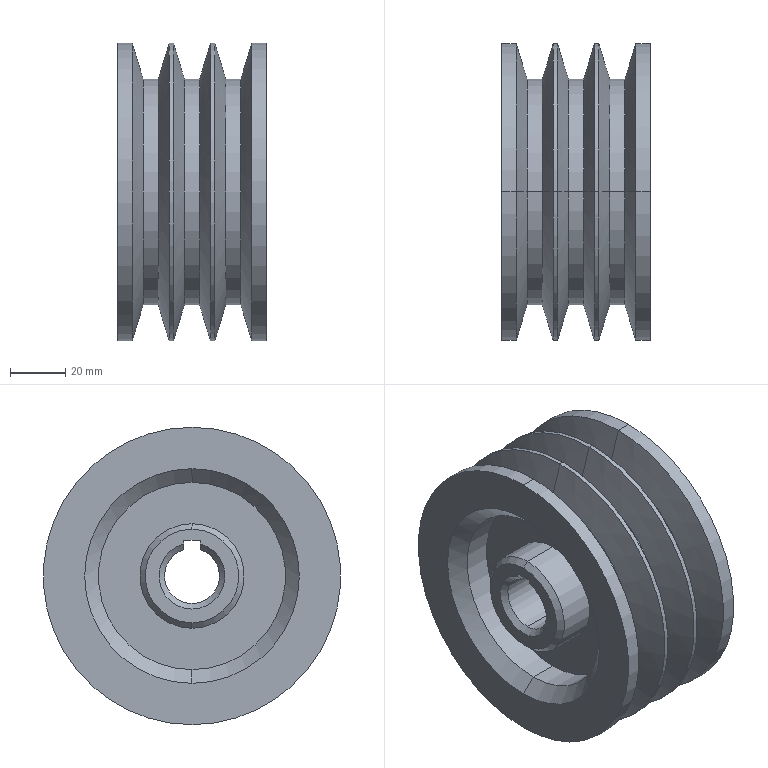Part | STEP file | Driven pulley | 1 solid | 54 faces | box 54 x 108 x 108 mm | volume 283345 mm3 | cylinder 24 | cone 21 | plane 9 | commonest cylinder face diameters 108 x8 82 x6 38 x4 68 x4 20 x2
STEP:
#1=CARTESIAN_POINT('',(17.5,0.,-10.));
#2=VERTEX_POINT('',#1);
#3=CARTESIAN_POINT('',(17.5,3.,9.539));
#4=VERTEX_POINT('',#3);
#5=CARTESIAN_POINT('',(17.5,0.,0.));
#6=DIRECTION('',(1.,0.,0.));
#7=DIRECTION('',(0.,0.,1.));
#8=AXIS2_PLACEMENT_3D('',#5,#6,#7);
#9=CIRCLE('',#8,10.);
#10=EDGE_CURVE('',#2,#4,#9,.T.);
#11=ORIENTED_EDGE('',*,*,#10,.F.);
#12=CARTESIAN_POINT('',(19.5,0.,-12.));
#13=VERTEX_POINT('',#12);
#14=CARTESIAN_POINT('',(17.5,0.,-10.));
#15=DIRECTION('',(0.7071,0.,-0.7071));
#16=VECTOR('',#15,1000.);
#17=LINE('',#14,#16);
#18=EDGE_CURVE('',#2,#13,#17,.T.);
#19=ORIENTED_EDGE('',*,*,#18,.T.);
#20=CARTESIAN_POINT('',(19.5,3.,11.619));
#21=VERTEX_POINT('',#20);
#22=CARTESIAN_POINT('',(19.5,0.,0.));
#23=DIRECTION('',(-1.,0.,0.));
#24=DIRECTION('',(0.,0.,1.));
#25=AXIS2_PLACEMENT_3D('',#22,#23,#24);
#26=CIRCLE('',#25,12.);
#27=EDGE_CURVE('',#21,#13,#26,.T.);
#28=ORIENTED_EDGE('',*,*,#27,.F.);
#29=CARTESIAN_POINT('',(17.5,3.,9.539));
#30=CARTESIAN_POINT('',(18.164,3.,10.235));
#31=CARTESIAN_POINT('',(18.831,3.,10.928));
#32=CARTESIAN_POINT('',(19.5,3.,11.619));
#33=B_SPLINE_CURVE_WITH_KNOTS('',3,(#29,#30,#31,#32),.UNSPECIFIED.,.F.,.F.,(4,4),(0.,0.002885),.UNSPECIFIED.);
#34=EDGE_CURVE('',#4,#21,#33,.T.);
#35=ORIENTED_EDGE('',*,*,#34,.F.);
#36=EDGE_LOOP('',(#11,#19,#28,#35));
#37=FACE_OUTER_BOUND('',#36,.T.);
#38=CARTESIAN_POINT('',(17.5,0.,0.));
#39=DIRECTION('',(1.,0.,0.));
#40=DIRECTION('',(0.,0.,-1.));
#41=AXIS2_PLACEMENT_3D('',#38,#39,#40);
#42=CONICAL_SURFACE('',#41,10.,0.7854);
#43=ADVANCED_FACE('',(#37),#42,.F.);
#44=CARTESIAN_POINT('',(-34.5,0.,17.));
#45=VERTEX_POINT('',#44);
#46=CARTESIAN_POINT('',(-34.5,0.,-17.));
#47=VERTEX_POINT('',#46);
#48=CARTESIAN_POINT('',(-34.5,0.,0.));
#49=DIRECTION('',(-1.,0.,0.));
#50=DIRECTION('',(0.,0.,-1.));
#51=AXIS2_PLACEMENT_3D('',#48,#49,#50);
#52=CIRCLE('',#51,17.);
#53=EDGE_CURVE('',#45,#47,#52,.T.);
#54=ORIENTED_EDGE('',*,*,#53,.F.);
#55=CARTESIAN_POINT('',(-32.5,0.,19.));
#56=VERTEX_POINT('',#55);
#57=CARTESIAN_POINT('',(-34.5,0.,17.));
#58=DIRECTION('',(0.7071,0.,0.7071));
#59=VECTOR('',#58,1000.);
#60=LINE('',#57,#59);
#61=EDGE_CURVE('',#45,#56,#60,.T.);
#62=ORIENTED_EDGE('',*,*,#61,.T.);
#63=CARTESIAN_POINT('',(-32.5,0.,-19.));
#64=VERTEX_POINT('',#63);
#65=CARTESIAN_POINT('',(-32.5,0.,0.));
#66=DIRECTION('',(1.,0.,0.));
#67=DIRECTION('',(0.,0.,-1.));
#68=AXIS2_PLACEMENT_3D('',#65,#66,#67);
#69=CIRCLE('',#68,19.);
#70=EDGE_CURVE('',#64,#56,#69,.T.);
#71=ORIENTED_EDGE('',*,*,#70,.F.);
#72=CARTESIAN_POINT('',(-34.5,0.,-17.));
#73=DIRECTION('',(0.7071,0.,-0.7071));
#74=VECTOR('',#73,1000.);
#75=LINE('',#72,#74);
#76=EDGE_CURVE('',#47,#64,#75,.T.);
#77=ORIENTED_EDGE('',*,*,#76,.F.);
#78=EDGE_LOOP('',(#54,#62,#71,#77));
#79=FACE_OUTER_BOUND('',#78,.T.);
#80=CARTESIAN_POINT('',(-34.5,0.,0.));
#81=DIRECTION('',(1.,0.,0.));
#82=DIRECTION('',(0.,0.,-1.));
#83=AXIS2_PLACEMENT_3D('',#80,#81,#82);
#84=CONICAL_SURFACE('',#83,17.,0.7854);
#85=ADVANCED_FACE('',(#79),#84,.T.);
#86=CARTESIAN_POINT('',(14.5,0.,34.));
#87=VERTEX_POINT('',#86);
#88=CARTESIAN_POINT('',(14.5,0.,-34.));
#89=VERTEX_POINT('',#88);
#90=CARTESIAN_POINT('',(14.5,0.,0.));
#91=DIRECTION('',(1.,0.,0.));
#92=DIRECTION('',(0.,0.,1.));
#93=AXIS2_PLACEMENT_3D('',#90,#91,#92);
#94=CIRCLE('',#93,34.);
#95=EDGE_CURVE('',#87,#89,#94,.T.);
#96=ORIENTED_EDGE('',*,*,#95,.F.);
#97=CARTESIAN_POINT('',(19.5,0.,39.));
#98=VERTEX_POINT('',#97);
#99=CARTESIAN_POINT('',(19.5,0.,39.));
#100=DIRECTION('',(0.7071,0.,0.7071));
#101=VECTOR('',#100,1000.);
#102=LINE('',#99,#101);
#103=EDGE_CURVE('',#87,#98,#102,.T.);
#104=ORIENTED_EDGE('',*,*,#103,.T.);
#105=CARTESIAN_POINT('',(19.5,0.,-39.));
#106=VERTEX_POINT('',#105);
#107=CARTESIAN_POINT('',(19.5,0.,0.));
#108=DIRECTION('',(-1.,0.,0.));
#109=DIRECTION('',(0.,0.,1.));
#110=AXIS2_PLACEMENT_3D('',#107,#108,#109);
#111=CIRCLE('',#110,39.);
#112=EDGE_CURVE('',#106,#98,#111,.T.);
#113=ORIENTED_EDGE('',*,*,#112,.F.);
#114=CARTESIAN_POINT('',(19.5,0.,-39.));
#115=DIRECTION('',(0.7071,0.,-0.7071));
#116=VECTOR('',#115,1000.);
#117=LINE('',#114,#116);
#118=EDGE_CURVE('',#89,#106,#117,.T.);
#119=ORIENTED_EDGE('',*,*,#118,.F.);
#120=EDGE_LOOP('',(#96,#104,#113,#119));
#121=FACE_OUTER_BOUND('',#120,.T.);
#122=CARTESIAN_POINT('',(19.5,0.,0.));
#123=DIRECTION('',(1.,0.,0.));
#124=DIRECTION('',(0.,0.,-1.));
#125=AXIS2_PLACEMENT_3D('',#122,#123,#124);
#126=CONICAL_SURFACE('',#125,39.,0.7854);
#127=ADVANCED_FACE('',(#121),#126,.F.);
#128=CARTESIAN_POINT('',(-29.5,0.,-34.));
#129=VERTEX_POINT('',#128);
#130=CARTESIAN_POINT('',(-29.5,0.,34.));
#131=VERTEX_POINT('',#130);
#132=CARTESIAN_POINT('',(-29.5,0.,0.));
#133=DIRECTION('',(-1.,0.,0.));
#134=DIRECTION('',(0.,0.,-1.));
#135=AXIS2_PLACEMENT_3D('',#132,#133,#134);
#136=CIRCLE('',#135,34.);
#137=EDGE_CURVE('',#129,#131,#136,.T.);
#138=ORIENTED_EDGE('',*,*,#137,.F.);
#139=CARTESIAN_POINT('',(-34.5,0.,-39.));
#140=VERTEX_POINT('',#139);
#141=CARTESIAN_POINT('',(-29.5,0.,-34.));
#142=DIRECTION('',(-0.7071,0.,-0.7071));
#143=VECTOR('',#142,1000.);
#144=LINE('',#141,#143);
#145=EDGE_CURVE('',#129,#140,#144,.T.);
#146=ORIENTED_EDGE('',*,*,#145,.T.);
#147=CARTESIAN_POINT('',(-34.5,0.,39.));
#148=VERTEX_POINT('',#147);
#149=CARTESIAN_POINT('',(-34.5,0.,0.));
#150=DIRECTION('',(1.,0.,0.));
#151=DIRECTION('',(0.,0.,-1.));
#152=AXIS2_PLACEMENT_3D('',#149,#150,#151);
#153=CIRCLE('',#152,39.);
#154=EDGE_CURVE('',#148,#140,#153,.T.);
#155=ORIENTED_EDGE('',*,*,#154,.F.);
#156=CARTESIAN_POINT('',(-29.5,0.,34.));
#157=DIRECTION('',(-0.7071,0.,0.7071));
#158=VECTOR('',#157,1000.);
#159=LINE('',#156,#158);
#160=EDGE_CURVE('',#131,#148,#159,.T.);
#161=ORIENTED_EDGE('',*,*,#160,.F.);
#162=EDGE_LOOP('',(#138,#146,#155,#161));
#163=FACE_OUTER_BOUND('',#162,.T.);
#164=CARTESIAN_POINT('',(-29.5,0.,0.));
#165=DIRECTION('',(-1.,0.,0.));
#166=DIRECTION('',(0.,0.,1.));
#167=AXIS2_PLACEMENT_3D('',#164,#165,#166);
#168=CONICAL_SURFACE('',#167,34.,0.7854);
#169=ADVANCED_FACE('',(#163),#168,.F.);
#170=CARTESIAN_POINT('',(4.5,0.,19.));
#171=VERTEX_POINT('',#170);
#172=CARTESIAN_POINT('',(4.5,0.,-19.));
#173=VERTEX_POINT('',#172);
#174=CARTESIAN_POINT('',(4.5,0.,0.));
#175=DIRECTION('',(-1.,0.,0.));
#176=DIRECTION('',(0.,0.,1.));
#177=AXIS2_PLACEMENT_3D('',#174,#175,#176);
#178=CIRCLE('',#177,19.);
#179=EDGE_CURVE('',#171,#173,#178,.T.);
#180=ORIENTED_EDGE('',*,*,#179,.F.);
#181=CARTESIAN_POINT('',(19.5,0.,19.));
#182=VERTEX_POINT('',#181);
#183=CARTESIAN_POINT('',(4.5,0.,19.));
#184=DIRECTION('',(1.,0.,0.));
#185=VECTOR('',#184,1000.);
#186=LINE('',#183,#185);
#187=EDGE_CURVE('',#171,#182,#186,.T.);
#188=ORIENTED_EDGE('',*,*,#187,.T.);
#189=CARTESIAN_POINT('',(19.5,0.,-19.));
#190=VERTEX_POINT('',#189);
#191=CARTESIAN_POINT('',(19.5,0.,0.));
#192=DIRECTION('',(-1.,0.,0.));
#193=DIRECTION('',(0.,0.,1.));
#194=AXIS2_PLACEMENT_3D('',#191,#192,#193);
#195=CIRCLE('',#194,19.);
#196=EDGE_CURVE('',#182,#190,#195,.T.);
#197=ORIENTED_EDGE('',*,*,#196,.T.);
#198=CARTESIAN_POINT('',(4.5,0.,-19.));
#199=DIRECTION('',(1.,0.,0.));
#200=VECTOR('',#199,1000.);
#201=LINE('',#198,#200);
#202=EDGE_CURVE('',#173,#190,#201,.T.);
#203=ORIENTED_EDGE('',*,*,#202,.F.);
#204=EDGE_LOOP('',(#180,#188,#197,#203));
#205=FACE_OUTER_BOUND('',#204,.T.);
#206=CARTESIAN_POINT('',(4.5,0.,0.));
#207=DIRECTION('',(1.,0.,0.));
#208=DIRECTION('',(0.,0.,-1.));
#209=AXIS2_PLACEMENT_3D('',#206,#207,#208);
#210=CYLINDRICAL_SURFACE('',#209,19.);
#211=ADVANCED_FACE('',(#205),#210,.T.);
#212=CARTESIAN_POINT('',(4.5,0.,-34.));
#213=VERTEX_POINT('',#212);
#214=CARTESIAN_POINT('',(4.5,0.,34.));
#215=VERTEX_POINT('',#214);
#216=CARTESIAN_POINT('',(4.5,0.,0.));
#217=DIRECTION('',(-1.,0.,0.));
#218=DIRECTION('',(0.,0.,1.));
#219=AXIS2_PLACEMENT_3D('',#216,#217,#218);
#220=CIRCLE('',#219,34.);
#221=EDGE_CURVE('',#213,#215,#220,.T.);
#222=ORIENTED_EDGE('',*,*,#221,.T.);
#223=CARTESIAN_POINT('',(4.5,0.,34.));
#224=DIRECTION('',(1.,0.,0.));
#225=VECTOR('',#224,1000.);
#226=LINE('',#223,#225);
#227=EDGE_CURVE('',#215,#87,#226,.T.);
#228=ORIENTED_EDGE('',*,*,#227,.T.);
#229=ORIENTED_EDGE('',*,*,#95,.T.);
#230=CARTESIAN_POINT('',(4.5,0.,-34.));
#231=DIRECTION('',(1.,0.,0.));
#232=VECTOR('',#231,1000.);
#233=LINE('',#230,#232);
#234=EDGE_CURVE('',#213,#89,#233,.T.);
#235=ORIENTED_EDGE('',*,*,#234,.F.);
#236=EDGE_LOOP('',(#222,#228,#229,#235));
#237=FACE_OUTER_BOUND('',#236,.T.);
#238=CARTESIAN_POINT('',(4.5,0.,0.));
#239=DIRECTION('',(1.,0.,0.));
#240=DIRECTION('',(0.,0.,-1.));
#241=AXIS2_PLACEMENT_3D('',#238,#239,#240);
#242=CYLINDRICAL_SURFACE('',#241,34.);
#243=ADVANCED_FACE('',(#237),#242,.F.);
#244=CARTESIAN_POINT('',(-19.5,0.,19.));
#245=VERTEX_POINT('',#244);
#246=CARTESIAN_POINT('',(-19.5,0.,-19.));
#247=VERTEX_POINT('',#246);
#248=CARTESIAN_POINT('',(-19.5,0.,0.));
#249=DIRECTION('',(-1.,0.,0.));
#250=DIRECTION('',(0.,0.,1.));
#251=AXIS2_PLACEMENT_3D('',#248,#249,#250);
#252=CIRCLE('',#251,19.);
#253=EDGE_CURVE('',#245,#247,#252,.T.);
#254=ORIENTED_EDGE('',*,*,#253,.T.);
#255=CARTESIAN_POINT('',(-19.5,0.,-19.));
#256=DIRECTION('',(-1.,0.,0.));
#257=VECTOR('',#256,1000.);
#258=LINE('',#255,#257);
#259=EDGE_CURVE('',#247,#64,#258,.T.);
#260=ORIENTED_EDGE('',*,*,#259,.T.);
#261=ORIENTED_EDGE('',*,*,#70,.T.);
#262=CARTESIAN_POINT('',(-19.5,0.,19.));
#263=DIRECTION('',(-1.,0.,0.));
#264=VECTOR('',#263,1000.);
#265=LINE('',#262,#264);
#266=EDGE_CURVE('',#245,#56,#265,.T.);
#267=ORIENTED_EDGE('',*,*,#266,.F.);
#268=EDGE_LOOP('',(#254,#260,#261,#267));
#269=FACE_OUTER_BOUND('',#268,.T.);
#270=CARTESIAN_POINT('',(-19.5,0.,0.));
#271=DIRECTION('',(-1.,0.,0.));
#272=DIRECTION('',(0.,0.,1.));
#273=AXIS2_PLACEMENT_3D('',#270,#271,#272);
#274=CYLINDRICAL_SURFACE('',#273,19.);
#275=ADVANCED_FACE('',(#269),#274,.T.);
#276=CARTESIAN_POINT('',(-19.5,0.,-34.));
#277=VERTEX_POINT('',#276);
#278=CARTESIAN_POINT('',(-19.5,0.,34.));
#279=VERTEX_POINT('',#278);
#280=CARTESIAN_POINT('',(-19.5,0.,0.));
#281=DIRECTION('',(-1.,0.,0.));
#282=DIRECTION('',(0.,0.,1.));
#283=AXIS2_PLACEMENT_3D('',#280,#281,#282);
#284=CIRCLE('',#283,34.);
#285=EDGE_CURVE('',#277,#279,#284,.T.);
#286=ORIENTED_EDGE('',*,*,#285,.F.);
#287=CARTESIAN_POINT('',(-19.5,0.,-34.));
#288=DIRECTION('',(-1.,0.,0.));
#289=VECTOR('',#288,1000.);
#290=LINE('',#287,#289);
#291=EDGE_CURVE('',#277,#129,#290,.T.);
#292=ORIENTED_EDGE('',*,*,#291,.T.);
#293=ORIENTED_EDGE('',*,*,#137,.T.);
#294=CARTESIAN_POINT('',(-19.5,0.,34.));
#295=DIRECTION('',(-1.,0.,0.));
#296=VECTOR('',#295,1000.);
#297=LINE('',#294,#296);
#298=EDGE_CURVE('',#279,#131,#297,.T.);
#299=ORIENTED_EDGE('',*,*,#298,.F.);
#300=EDGE_LOOP('',(#286,#292,#293,#299));
#301=FACE_OUTER_BOUND('',#300,.T.);
#302=CARTESIAN_POINT('',(-19.5,0.,0.));
#303=DIRECTION('',(-1.,0.,0.));
#304=DIRECTION('',(0.,0.,1.));
#305=AXIS2_PLACEMENT_3D('',#302,#303,#304);
#306=CYLINDRICAL_SURFACE('',#305,34.);
#307=ADVANCED_FACE('',(#301),#306,.F.);
#308=CARTESIAN_POINT('',(-32.5,3.,9.539));
#309=VERTEX_POINT('',#308);
#310=CARTESIAN_POINT('',(-32.5,0.,-10.));
#311=VERTEX_POINT('',#310);
#312=CARTESIAN_POINT('',(-32.5,0.,0.));
#313=DIRECTION('',(-1.,0.,0.));
#314=DIRECTION('',(0.,0.,-1.));
#315=AXIS2_PLACEMENT_3D('',#312,#313,#314);
#316=CIRCLE('',#315,10.);
#317=EDGE_CURVE('',#309,#311,#316,.T.);
#318=ORIENTED_EDGE('',*,*,#317,.T.);
#319=CARTESIAN_POINT('',(-59.5,0.,-10.));
#320=DIRECTION('',(1.,0.,0.));
#321=VECTOR('',#320,1000.);
#322=LINE('',#319,#321);
#323=EDGE_CURVE('',#311,#2,#322,.T.);
#324=ORIENTED_EDGE('',*,*,#323,.T.);
#325=ORIENTED_EDGE('',*,*,#10,.T.);
#326=CARTESIAN_POINT('',(-59.5,3.,9.539));
#327=DIRECTION('',(-1.,0.,0.));
#328=VECTOR('',#327,1000.);
#329=LINE('',#326,#328);
#330=EDGE_CURVE('',#4,#309,#329,.T.);
#331=ORIENTED_EDGE('',*,*,#330,.T.);
#332=EDGE_LOOP('',(#318,#324,#325,#331));
#333=FACE_OUTER_BOUND('',#332,.T.);
#334=CARTESIAN_POINT('',(-59.5,0.,0.));
#335=DIRECTION('',(1.,0.,0.));
#336=DIRECTION('',(0.,0.,-1.));
#337=AXIS2_PLACEMENT_3D('',#334,#335,#336);
#338=CYLINDRICAL_SURFACE('',#337,10.);
#339=ADVANCED_FACE('',(#333),#338,.F.);
#340=CARTESIAN_POINT('',(19.5,0.,54.));
#341=VERTEX_POINT('',#340);
#342=CARTESIAN_POINT('',(19.5,0.,-54.));
#343=VERTEX_POINT('',#342);
#344=CARTESIAN_POINT('',(19.5,0.,0.));
#345=DIRECTION('',(-1.,0.,0.));
#346=DIRECTION('',(0.,0.,1.));
#347=AXIS2_PLACEMENT_3D('',#344,#345,#346);
#348=CIRCLE('',#347,54.);
#349=EDGE_CURVE('',#341,#343,#348,.T.);
#350=ORIENTED_EDGE('',*,*,#349,.T.);
#351=CARTESIAN_POINT('',(14.223,0.,-54.));
#352=VERTEX_POINT('',#351);
#353=CARTESIAN_POINT('',(0.,0.,-54.));
#354=DIRECTION('',(-1.,0.,0.));
#355=VECTOR('',#354,1000.);
#356=LINE('',#353,#355);
#357=EDGE_CURVE('',#343,#352,#356,.T.);
#358=ORIENTED_EDGE('',*,*,#357,.T.);
#359=CARTESIAN_POINT('',(14.223,0.,54.));
#360=VERTEX_POINT('',#359);
#361=CARTESIAN_POINT('',(14.223,0.,0.));
#362=DIRECTION('',(-1.,0.,0.));
#363=DIRECTION('',(0.,0.,1.));
#364=AXIS2_PLACEMENT_3D('',#361,#362,#363);
#365=CIRCLE('',#364,54.);
#366=EDGE_CURVE('',#360,#352,#365,.T.);
#367=ORIENTED_EDGE('',*,*,#366,.F.);
#368=CARTESIAN_POINT('',(0.,0.,54.));
#369=DIRECTION('',(-1.,0.,0.));
#370=VECTOR('',#369,1000.);
#371=LINE('',#368,#370);
#372=EDGE_CURVE('',#341,#360,#371,.T.);
#373=ORIENTED_EDGE('',*,*,#372,.F.);
#374=EDGE_LOOP('',(#350,#358,#367,#373));
#375=FACE_OUTER_BOUND('',#374,.T.);
#376=CARTESIAN_POINT('',(0.,0.,0.));
#377=DIRECTION('',(-1.,0.,0.));
#378=DIRECTION('',(0.,0.,1.));
#379=AXIS2_PLACEMENT_3D('',#376,#377,#378);
#380=CYLINDRICAL_SURFACE('',#379,54.);
#381=ADVANCED_FACE('',(#375),#380,.T.);
#382=CARTESIAN_POINT('',(10.248,0.,41.));
#383=VERTEX_POINT('',#382);
#384=CARTESIAN_POINT('',(10.248,0.,-41.));
#385=VERTEX_POINT('',#384);
#386=CARTESIAN_POINT('',(10.248,0.,0.));
#387=DIRECTION('',(-1.,0.,0.));
#388=DIRECTION('',(0.,0.,1.));
#389=AXIS2_PLACEMENT_3D('',#386,#387,#388);
#390=CIRCLE('',#389,41.);
#391=EDGE_CURVE('',#383,#385,#390,.T.);
#392=ORIENTED_EDGE('',*,*,#391,.F.);
#393=CARTESIAN_POINT('',(14.223,0.,54.));
#394=DIRECTION('',(0.2924,0.,0.9563));
#395=VECTOR('',#394,1000.);
#396=LINE('',#393,#395);
#397=EDGE_CURVE('',#383,#360,#396,.T.);
#398=ORIENTED_EDGE('',*,*,#397,.T.);
#399=ORIENTED_EDGE('',*,*,#366,.T.);
#400=CARTESIAN_POINT('',(14.223,0.,-54.));
#401=DIRECTION('',(0.2924,0.,-0.9563));
#402=VECTOR('',#401,1000.);
#403=LINE('',#400,#402);
#404=EDGE_CURVE('',#385,#352,#403,.T.);
#405=ORIENTED_EDGE('',*,*,#404,.F.);
#406=EDGE_LOOP('',(#392,#398,#399,#405));
#407=FACE_OUTER_BOUND('',#406,.T.);
#408=CARTESIAN_POINT('',(14.223,0.,0.));
#409=DIRECTION('',(1.,0.,0.));
#410=DIRECTION('',(0.,0.,-1.));
#411=AXIS2_PLACEMENT_3D('',#408,#409,#410);
#412=CONICAL_SURFACE('',#411,54.,1.274);
#413=ADVANCED_FACE('',(#407),#412,.T.);
#414=ORIENTED_EDGE('',*,*,#391,.T.);
#415=CARTESIAN_POINT('',(4.752,0.,-41.));
#416=VERTEX_POINT('',#415);
#417=CARTESIAN_POINT('',(0.,0.,-41.));
#418=DIRECTION('',(-1.,0.,0.));
#419=VECTOR('',#418,1000.);
#420=LINE('',#417,#419);
#421=EDGE_CURVE('',#385,#416,#420,.T.);
#422=ORIENTED_EDGE('',*,*,#421,.T.);
#423=CARTESIAN_POINT('',(4.752,0.,41.));
#424=VERTEX_POINT('',#423);
#425=CARTESIAN_POINT('',(4.752,0.,0.));
#426=DIRECTION('',(-1.,0.,0.));
#427=DIRECTION('',(0.,0.,1.));
#428=AXIS2_PLACEMENT_3D('',#425,#426,#427);
#429=CIRCLE('',#428,41.);
#430=EDGE_CURVE('',#424,#416,#429,.T.);
#431=ORIENTED_EDGE('',*,*,#430,.F.);
#432=CARTESIAN_POINT('',(0.,0.,41.));
#433=DIRECTION('',(-1.,0.,0.));
#434=VECTOR('',#433,1000.);
#435=LINE('',#432,#434);
#436=EDGE_CURVE('',#383,#424,#435,.T.);
#437=ORIENTED_EDGE('',*,*,#436,.F.);
#438=EDGE_LOOP('',(#414,#422,#431,#437));
#439=FACE_OUTER_BOUND('',#438,.T.);
#440=CARTESIAN_POINT('',(0.,0.,0.));
#441=DIRECTION('',(-1.,0.,0.));
#442=DIRECTION('',(0.,0.,1.));
#443=AXIS2_PLACEMENT_3D('',#440,#441,#442);
#444=CYLINDRICAL_SURFACE('',#443,41.);
#445=ADVANCED_FACE('',(#439),#444,.T.);
#446=ORIENTED_EDGE('',*,*,#430,.T.);
#447=CARTESIAN_POINT('',(0.7771,0.,-54.));
#448=VERTEX_POINT('',#447);
#449=CARTESIAN_POINT('',(4.752,0.,-41.));
#450=DIRECTION('',(-0.2924,0.,-0.9563));
#451=VECTOR('',#450,1000.);
#452=LINE('',#449,#451);
#453=EDGE_CURVE('',#416,#448,#452,.T.);
#454=ORIENTED_EDGE('',*,*,#453,.T.);
#455=CARTESIAN_POINT('',(0.7771,0.,54.));
#456=VERTEX_POINT('',#455);
#457=CARTESIAN_POINT('',(0.7771,0.,0.));
#458=DIRECTION('',(-1.,0.,0.));
#459=DIRECTION('',(0.,0.,1.));
#460=AXIS2_PLACEMENT_3D('',#457,#458,#459);
#461=CIRCLE('',#460,54.);
#462=EDGE_CURVE('',#456,#448,#461,.T.);
#463=ORIENTED_EDGE('',*,*,#462,.F.);
#464=CARTESIAN_POINT('',(4.752,0.,41.));
#465=DIRECTION('',(-0.2924,0.,0.9563));
#466=VECTOR('',#465,1000.);
#467=LINE('',#464,#466);
#468=EDGE_CURVE('',#424,#456,#467,.T.);
#469=ORIENTED_EDGE('',*,*,#468,.F.);
#470=EDGE_LOOP('',(#446,#454,#463,#469));
#471=FACE_OUTER_BOUND('',#470,.T.);
#472=CARTESIAN_POINT('',(4.752,0.,0.));
#473=DIRECTION('',(-1.,0.,0.));
#474=DIRECTION('',(0.,0.,1.));
#475=AXIS2_PLACEMENT_3D('',#472,#473,#474);
#476=CONICAL_SURFACE('',#475,41.,1.274);
#477=ADVANCED_FACE('',(#471),#476,.T.);
#478=ORIENTED_EDGE('',*,*,#462,.T.);
#479=CARTESIAN_POINT('',(-0.7771,0.,-54.));
#480=VERTEX_POINT('',#479);
#481=CARTESIAN_POINT('',(0.,0.,-54.));
#482=DIRECTION('',(-1.,0.,0.));
#483=VECTOR('',#482,1000.);
#484=LINE('',#481,#483);
#485=EDGE_CURVE('',#448,#480,#484,.T.);
#486=ORIENTED_EDGE('',*,*,#485,.T.);
#487=CARTESIAN_POINT('',(-0.7771,0.,54.));
#488=VERTEX_POINT('',#487);
#489=CARTESIAN_POINT('',(-0.7771,0.,0.));
#490=DIRECTION('',(-1.,0.,0.));
#491=DIRECTION('',(0.,0.,1.));
#492=AXIS2_PLACEMENT_3D('',#489,#490,#491);
#493=CIRCLE('',#492,54.);
#494=EDGE_CURVE('',#488,#480,#493,.T.);
#495=ORIENTED_EDGE('',*,*,#494,.F.);
#496=CARTESIAN_POINT('',(0.,0.,54.));
#497=DIRECTION('',(-1.,0.,0.));
#498=VECTOR('',#497,1000.);
#499=LINE('',#496,#498);
#500=EDGE_CURVE('',#456,#488,#499,.T.);
#501=ORIENTED_EDGE('',*,*,#500,.F.);
#502=EDGE_LOOP('',(#478,#486,#495,#501));
#503=FACE_OUTER_BOUND('',#502,.T.);
#504=CARTESIAN_POINT('',(0.,0.,0.));
#505=DIRECTION('',(-1.,0.,0.));
#506=DIRECTION('',(0.,0.,1.));
#507=AXIS2_PLACEMENT_3D('',#504,#505,#506);
#508=CYLINDRICAL_SURFACE('',#507,54.);
#509=ADVANCED_FACE('',(#503),#508,.T.);
#510=CARTESIAN_POINT('',(-4.752,0.,41.));
#511=VERTEX_POINT('',#510);
#512=CARTESIAN_POINT('',(-4.752,0.,-41.));
#513=VERTEX_POINT('',#512);
#514=CARTESIAN_POINT('',(-4.752,0.,0.));
#515=DIRECTION('',(-1.,0.,0.));
#516=DIRECTION('',(0.,0.,1.));
#517=AXIS2_PLACEMENT_3D('',#514,#515,#516);
#518=CIRCLE('',#517,41.);
#519=EDGE_CURVE('',#511,#513,#518,.T.);
#520=ORIENTED_EDGE('',*,*,#519,.F.);
#521=CARTESIAN_POINT('',(-0.7771,0.,54.));
#522=DIRECTION('',(0.2924,0.,0.9563));
#523=VECTOR('',#522,1000.);
#524=LINE('',#521,#523);
#525=EDGE_CURVE('',#511,#488,#524,.T.);
#526=ORIENTED_EDGE('',*,*,#525,.T.);
#527=ORIENTED_EDGE('',*,*,#494,.T.);
#528=CARTESIAN_POINT('',(-0.7771,0.,-54.));
#529=DIRECTION('',(0.2924,0.,-0.9563));
#530=VECTOR('',#529,1000.);
#531=LINE('',#528,#530);
#532=EDGE_CURVE('',#513,#480,#531,.T.);
#533=ORIENTED_EDGE('',*,*,#532,.F.);
#534=EDGE_LOOP('',(#520,#526,#527,#533));
#535=FACE_OUTER_BOUND('',#534,.T.);
#536=CARTESIAN_POINT('',(-0.7771,0.,0.));
#537=DIRECTION('',(1.,0.,0.));
#538=DIRECTION('',(0.,0.,-1.));
#539=AXIS2_PLACEMENT_3D('',#536,#537,#538);
#540=CONICAL_SURFACE('',#539,54.,1.274);
#541=ADVANCED_FACE('',(#535),#540,.T.);
#542=ORIENTED_EDGE('',*,*,#519,.T.);
#543=CARTESIAN_POINT('',(-10.248,0.,-41.));
#544=VERTEX_POINT('',#543);
#545=CARTESIAN_POINT('',(0.,0.,-41.));
#546=DIRECTION('',(-1.,0.,0.));
#547=VECTOR('',#546,1000.);
#548=LINE('',#545,#547);
#549=EDGE_CURVE('',#513,#544,#548,.T.);
#550=ORIENTED_EDGE('',*,*,#549,.T.);
#551=CARTESIAN_POINT('',(-10.248,0.,41.));
#552=VERTEX_POINT('',#551);
#553=CARTESIAN_POINT('',(-10.248,0.,0.));
#554=DIRECTION('',(-1.,0.,0.));
#555=DIRECTION('',(0.,0.,1.));
#556=AXIS2_PLACEMENT_3D('',#553,#554,#555);
#557=CIRCLE('',#556,41.);
#558=EDGE_CURVE('',#552,#544,#557,.T.);
#559=ORIENTED_EDGE('',*,*,#558,.F.);
#560=CARTESIAN_POINT('',(0.,0.,41.));
#561=DIRECTION('',(-1.,0.,0.));
#562=VECTOR('',#561,1000.);
#563=LINE('',#560,#562);
#564=EDGE_CURVE('',#511,#552,#563,.T.);
#565=ORIENTED_EDGE('',*,*,#564,.F.);
#566=EDGE_LOOP('',(#542,#550,#559,#565));
#567=FACE_OUTER_BOUND('',#566,.T.);
#568=CARTESIAN_POINT('',(0.,0.,0.));
#569=DIRECTION('',(-1.,0.,0.));
#570=DIRECTION('',(0.,0.,1.));
#571=AXIS2_PLACEMENT_3D('',#568,#569,#570);
#572=CYLINDRICAL_SURFACE('',#571,41.);
#573=ADVANCED_FACE('',(#567),#572,.T.);
#574=ORIENTED_EDGE('',*,*,#558,.T.);
#575=CARTESIAN_POINT('',(-14.223,0.,-54.));
#576=VERTEX_POINT('',#575);
#577=CARTESIAN_POINT('',(-10.248,0.,-41.));
#578=DIRECTION('',(-0.2924,0.,-0.9563));
#579=VECTOR('',#578,1000.);
#580=LINE('',#577,#579);
#581=EDGE_CURVE('',#544,#576,#580,.T.);
#582=ORIENTED_EDGE('',*,*,#581,.T.);
#583=CARTESIAN_POINT('',(-14.223,0.,54.));
#584=VERTEX_POINT('',#583);
#585=CARTESIAN_POINT('',(-14.223,0.,0.));
#586=DIRECTION('',(-1.,0.,0.));
#587=DIRECTION('',(0.,0.,1.));
#588=AXIS2_PLACEMENT_3D('',#585,#586,#587);
#589=CIRCLE('',#588,54.);
#590=EDGE_CURVE('',#584,#576,#589,.T.);
#591=ORIENTED_EDGE('',*,*,#590,.F.);
#592=CARTESIAN_POINT('',(-10.248,0.,41.));
#593=DIRECTION('',(-0.2924,0.,0.9563));
#594=VECTOR('',#593,1000.);
#595=LINE('',#592,#594);
#596=EDGE_CURVE('',#552,#584,#595,.T.);
#597=ORIENTED_EDGE('',*,*,#596,.F.);
#598=EDGE_LOOP('',(#574,#582,#591,#597));
#599=FACE_OUTER_BOUND('',#598,.T.);
#600=CARTESIAN_POINT('',(-10.248,0.,0.));
#601=DIRECTION('',(-1.,0.,0.));
#602=DIRECTION('',(0.,0.,1.));
#603=AXIS2_PLACEMENT_3D('',#600,#601,#602);
#604=CONICAL_SURFACE('',#603,41.,1.274);
#605=ADVANCED_FACE('',(#599),#604,.T.);
#606=ORIENTED_EDGE('',*,*,#590,.T.);
#607=CARTESIAN_POINT('',(-15.777,0.,-54.));
#608=VERTEX_POINT('',#607);
#609=CARTESIAN_POINT('',(0.,0.,-54.));
#610=DIRECTION('',(-1.,0.,0.));
#611=VECTOR('',#610,1000.);
#612=LINE('',#609,#611);
#613=EDGE_CURVE('',#576,#608,#612,.T.);
#614=ORIENTED_EDGE('',*,*,#613,.T.);
#615=CARTESIAN_POINT('',(-15.777,0.,54.));
#616=VERTEX_POINT('',#615);
#617=CARTESIAN_POINT('',(-15.777,0.,0.));
#618=DIRECTION('',(-1.,0.,0.));
#619=DIRECTION('',(0.,0.,1.));
#620=AXIS2_PLACEMENT_3D('',#617,#618,#619);
#621=CIRCLE('',#620,54.);
#622=EDGE_CURVE('',#616,#608,#621,.T.);
#623=ORIENTED_EDGE('',*,*,#622,.F.);
#624=CARTESIAN_POINT('',(0.,0.,54.));
#625=DIRECTION('',(-1.,0.,0.));
#626=VECTOR('',#625,1000.);
#627=LINE('',#624,#626);
#628=EDGE_CURVE('',#584,#616,#627,.T.);
#629=ORIENTED_EDGE('',*,*,#628,.F.);
#630=EDGE_LOOP('',(#606,#614,#623,#629));
#631=FACE_OUTER_BOUND('',#630,.T.);
#632=CARTESIAN_POINT('',(0.,0.,0.));
#633=DIRECTION('',(-1.,0.,0.));
#634=DIRECTION('',(0.,0.,1.));
#635=AXIS2_PLACEMENT_3D('',#632,#633,#634);
#636=CYLINDRICAL_SURFACE('',#635,54.);
#637=ADVANCED_FACE('',(#631),#636,.T.);
#638=CARTESIAN_POINT('',(-19.752,0.,41.));
#639=VERTEX_POINT('',#638);
#640=CARTESIAN_POINT('',(-19.752,0.,-41.));
#641=VERTEX_POINT('',#640);
#642=CARTESIAN_POINT('',(-19.752,0.,0.));
#643=DIRECTION('',(-1.,0.,0.));
#644=DIRECTION('',(0.,0.,1.));
#645=AXIS2_PLACEMENT_3D('',#642,#643,#644);
#646=CIRCLE('',#645,41.);
#647=EDGE_CURVE('',#639,#641,#646,.T.);
#648=ORIENTED_EDGE('',*,*,#647,.F.);
#649=CARTESIAN_POINT('',(-15.777,0.,54.));
#650=DIRECTION('',(0.2924,0.,0.9563));
#651=VECTOR('',#650,1000.);
#652=LINE('',#649,#651);
#653=EDGE_CURVE('',#639,#616,#652,.T.);
#654=ORIENTED_EDGE('',*,*,#653,.T.);
#655=ORIENTED_EDGE('',*,*,#622,.T.);
#656=CARTESIAN_POINT('',(-15.777,0.,-54.));
#657=DIRECTION('',(0.2924,0.,-0.9563));
#658=VECTOR('',#657,1000.);
#659=LINE('',#656,#658);
#660=EDGE_CURVE('',#641,#608,#659,.T.);
#661=ORIENTED_EDGE('',*,*,#660,.F.);
#662=EDGE_LOOP('',(#648,#654,#655,#661));
#663=FACE_OUTER_BOUND('',#662,.T.);
#664=CARTESIAN_POINT('',(-15.777,0.,0.));
#665=DIRECTION('',(1.,0.,0.));
#666=DIRECTION('',(0.,0.,-1.));
#667=AXIS2_PLACEMENT_3D('',#664,#665,#666);
#668=CONICAL_SURFACE('',#667,54.,1.274);
#669=ADVANCED_FACE('',(#663),#668,.T.);
#670=ORIENTED_EDGE('',*,*,#647,.T.);
#671=CARTESIAN_POINT('',(-25.248,0.,-41.));
#672=VERTEX_POINT('',#671);
#673=CARTESIAN_POINT('',(0.,0.,-41.));
#674=DIRECTION('',(-1.,0.,0.));
#675=VECTOR('',#674,1000.);
#676=LINE('',#673,#675);
#677=EDGE_CURVE('',#641,#672,#676,.T.);
#678=ORIENTED_EDGE('',*,*,#677,.T.);
#679=CARTESIAN_POINT('',(-25.248,0.,41.));
#680=VERTEX_POINT('',#679);
#681=CARTESIAN_POINT('',(-25.248,0.,0.));
#682=DIRECTION('',(-1.,0.,0.));
#683=DIRECTION('',(0.,0.,1.));
#684=AXIS2_PLACEMENT_3D('',#681,#682,#683);
#685=CIRCLE('',#684,41.);
#686=EDGE_CURVE('',#680,#672,#685,.T.);
#687=ORIENTED_EDGE('',*,*,#686,.F.);
#688=CARTESIAN_POINT('',(0.,0.,41.));
#689=DIRECTION('',(-1.,0.,0.));
#690=VECTOR('',#689,1000.);
#691=LINE('',#688,#690);
#692=EDGE_CURVE('',#639,#680,#691,.T.);
#693=ORIENTED_EDGE('',*,*,#692,.F.);
#694=EDGE_LOOP('',(#670,#678,#687,#693));
#695=FACE_OUTER_BOUND('',#694,.T.);
#696=CARTESIAN_POINT('',(0.,0.,0.));
#697=DIRECTION('',(-1.,0.,0.));
#698=DIRECTION('',(0.,0.,1.));
#699=AXIS2_PLACEMENT_3D('',#696,#697,#698);
#700=CYLINDRICAL_SURFACE('',#699,41.);
#701=ADVANCED_FACE('',(#695),#700,.T.);
#702=ORIENTED_EDGE('',*,*,#686,.T.);
#703=CARTESIAN_POINT('',(-29.223,0.,-54.));
#704=VERTEX_POINT('',#703);
#705=CARTESIAN_POINT('',(-25.248,0.,-41.));
#706=DIRECTION('',(-0.2924,0.,-0.9563));
#707=VECTOR('',#706,1000.);
#708=LINE('',#705,#707);
#709=EDGE_CURVE('',#672,#704,#708,.T.);
#710=ORIENTED_EDGE('',*,*,#709,.T.);
#711=CARTESIAN_POINT('',(-29.223,0.,54.));
#712=VERTEX_POINT('',#711);
#713=CARTESIAN_POINT('',(-29.223,0.,0.));
#714=DIRECTION('',(-1.,0.,0.));
#715=DIRECTION('',(0.,0.,1.));
#716=AXIS2_PLACEMENT_3D('',#713,#714,#715);
#717=CIRCLE('',#716,54.);
#718=EDGE_CURVE('',#712,#704,#717,.T.);
#719=ORIENTED_EDGE('',*,*,#718,.F.);
#720=CARTESIAN_POINT('',(-25.248,0.,41.));
#721=DIRECTION('',(-0.2924,0.,0.9563));
#722=VECTOR('',#721,1000.);
#723=LINE('',#720,#722);
#724=EDGE_CURVE('',#680,#712,#723,.T.);
#725=ORIENTED_EDGE('',*,*,#724,.F.);
#726=EDGE_LOOP('',(#702,#710,#719,#725));
#727=FACE_OUTER_BOUND('',#726,.T.);
#728=CARTESIAN_POINT('',(-25.248,0.,0.));
#729=DIRECTION('',(-1.,0.,0.));
#730=DIRECTION('',(0.,0.,1.));
#731=AXIS2_PLACEMENT_3D('',#728,#729,#730);
#732=CONICAL_SURFACE('',#731,41.,1.274);
#733=ADVANCED_FACE('',(#727),#732,.T.);
#734=ORIENTED_EDGE('',*,*,#718,.T.);
#735=CARTESIAN_POINT('',(-34.5,0.,-54.));
#736=VERTEX_POINT('',#735);
#737=CARTESIAN_POINT('',(0.,0.,-54.));
#738=DIRECTION('',(-1.,0.,0.));
#739=VECTOR('',#738,1000.);
#740=LINE('',#737,#739);
#741=EDGE_CURVE('',#704,#736,#740,.T.);
#742=ORIENTED_EDGE('',*,*,#741,.T.);
#743=CARTESIAN_POINT('',(-34.5,0.,54.));
#744=VERTEX_POINT('',#743);
#745=CARTESIAN_POINT('',(-34.5,0.,0.));
#746=DIRECTION('',(-1.,0.,0.));
#747=DIRECTION('',(0.,0.,1.));
#748=AXIS2_PLACEMENT_3D('',#745,#746,#747);
#749=CIRCLE('',#748,54.);
#750=EDGE_CURVE('',#744,#736,#749,.T.);
#751=ORIENTED_EDGE('',*,*,#750,.F.);
#752=CARTESIAN_POINT('',(0.,0.,54.));
#753=DIRECTION('',(-1.,0.,0.));
#754=VECTOR('',#753,1000.);
#755=LINE('',#752,#754);
#756=EDGE_CURVE('',#712,#744,#755,.T.);
#757=ORIENTED_EDGE('',*,*,#756,.F.);
#758=EDGE_LOOP('',(#734,#742,#751,#757));
#759=FACE_OUTER_BOUND('',#758,.T.);
#760=CARTESIAN_POINT('',(0.,0.,0.));
#761=DIRECTION('',(-1.,0.,0.));
#762=DIRECTION('',(0.,0.,1.));
#763=AXIS2_PLACEMENT_3D('',#760,#761,#762);
#764=CYLINDRICAL_SURFACE('',#763,54.);
#765=ADVANCED_FACE('',(#759),#764,.T.);
#766=CARTESIAN_POINT('',(19.5,3.,13.));
#767=VERTEX_POINT('',#766);
#768=CARTESIAN_POINT('',(19.5,3.,13.));
#769=DIRECTION('',(0.,0.,1.));
#770=VECTOR('',#769,1000.);
#771=LINE('',#768,#770);
#772=EDGE_CURVE('',#21,#767,#771,.T.);
#773=ORIENTED_EDGE('',*,*,#772,.F.);
#774=ORIENTED_EDGE('',*,*,#27,.T.);
#775=CARTESIAN_POINT('',(19.5,-3.,11.619));
#776=VERTEX_POINT('',#775);
#777=CARTESIAN_POINT('',(19.5,0.,0.));
#778=DIRECTION('',(-1.,0.,0.));
#779=DIRECTION('',(0.,0.,1.));
#780=AXIS2_PLACEMENT_3D('',#777,#778,#779);
#781=CIRCLE('',#780,12.);
#782=EDGE_CURVE('',#13,#776,#781,.T.);
#783=ORIENTED_EDGE('',*,*,#782,.T.);
#784=CARTESIAN_POINT('',(19.5,-3.,13.));
#785=VERTEX_POINT('',#784);
#786=CARTESIAN_POINT('',(19.5,-3.,13.));
#787=DIRECTION('',(0.,0.,-1.));
#788=VECTOR('',#787,1000.);
#789=LINE('',#786,#788);
#790=EDGE_CURVE('',#785,#776,#789,.T.);
#791=ORIENTED_EDGE('',*,*,#790,.F.);
#792=CARTESIAN_POINT('',(19.5,-3.,13.));
#793=DIRECTION('',(0.,-1.,0.));
#794=VECTOR('',#793,1000.);
#795=LINE('',#792,#794);
#796=EDGE_CURVE('',#767,#785,#795,.T.);
#797=ORIENTED_EDGE('',*,*,#796,.F.);
#798=EDGE_LOOP('',(#773,#774,#783,#791,#797));
#799=FACE_BOUND('',#798,.T.);
#800=CARTESIAN_POINT('',(19.5,0.,0.));
#801=DIRECTION('',(-1.,0.,0.));
#802=DIRECTION('',(0.,0.,1.));
#803=AXIS2_PLACEMENT_3D('',#800,#801,#802);
#804=CIRCLE('',#803,19.);
#805=EDGE_CURVE('',#190,#182,#804,.T.);
#806=ORIENTED_EDGE('',*,*,#805,.F.);
#807=ORIENTED_EDGE('',*,*,#196,.F.);
#808=EDGE_LOOP('',(#806,#807));
#809=FACE_OUTER_BOUND('',#808,.T.);
#810=CARTESIAN_POINT('',(19.5,54.,0.));
#811=DIRECTION('',(-1.,0.,0.));
#812=DIRECTION('',(0.,0.,1.));
#813=AXIS2_PLACEMENT_3D('',#810,#811,#812);
#814=PLANE('',#813);
#815=ADVANCED_FACE('',(#799,#809),#814,.F.);
#816=CARTESIAN_POINT('',(-34.5,0.,0.));
#817=DIRECTION('',(-1.,0.,0.));
#818=DIRECTION('',(0.,0.,-1.));
#819=AXIS2_PLACEMENT_3D('',#816,#817,#818);
#820=CIRCLE('',#819,17.);
#821=EDGE_CURVE('',#47,#45,#820,.T.);
#822=ORIENTED_EDGE('',*,*,#821,.T.);
#823=ORIENTED_EDGE('',*,*,#53,.T.);
#824=EDGE_LOOP('',(#822,#823));
#825=FACE_OUTER_BOUND('',#824,.T.);
#826=CARTESIAN_POINT('',(-34.5,-3.,13.));
#827=VERTEX_POINT('',#826);
#828=CARTESIAN_POINT('',(-34.5,-3.,11.619));
#829=VERTEX_POINT('',#828);
#830=CARTESIAN_POINT('',(-34.5,-3.,0.));
#831=DIRECTION('',(0.,0.,-1.));
#832=VECTOR('',#831,1000.);
#833=LINE('',#830,#832);
#834=EDGE_CURVE('',#827,#829,#833,.T.);
#835=ORIENTED_EDGE('',*,*,#834,.T.);
#836=CARTESIAN_POINT('',(-34.5,3.,11.619));
#837=VERTEX_POINT('',#836);
#838=CARTESIAN_POINT('',(-34.5,0.,0.));
#839=DIRECTION('',(1.,0.,0.));
#840=DIRECTION('',(0.,0.,-1.));
#841=AXIS2_PLACEMENT_3D('',#838,#839,#840);
#842=CIRCLE('',#841,12.);
#843=EDGE_CURVE('',#829,#837,#842,.T.);
#844=ORIENTED_EDGE('',*,*,#843,.T.);
#845=CARTESIAN_POINT('',(-34.5,3.,13.));
#846=VERTEX_POINT('',#845);
#847=CARTESIAN_POINT('',(-34.5,3.,0.));
#848=DIRECTION('',(0.,0.,1.));
#849=VECTOR('',#848,1000.);
#850=LINE('',#847,#849);
#851=EDGE_CURVE('',#837,#846,#850,.T.);
#852=ORIENTED_EDGE('',*,*,#851,.T.);
#853=CARTESIAN_POINT('',(-34.5,54.,13.));
#854=DIRECTION('',(0.,-1.,0.));
#855=VECTOR('',#854,1000.);
#856=LINE('',#853,#855);
#857=EDGE_CURVE('',#846,#827,#856,.T.);
#858=ORIENTED_EDGE('',*,*,#857,.T.);
#859=EDGE_LOOP('',(#835,#844,#852,#858));
#860=FACE_BOUND('',#859,.T.);
#861=CARTESIAN_POINT('',(-34.5,54.,0.));
#862=DIRECTION('',(1.,0.,0.));
#863=DIRECTION('',(0.,0.,-1.));
#864=AXIS2_PLACEMENT_3D('',#861,#862,#863);
#865=PLANE('',#864);
#866=ADVANCED_FACE('',(#825,#860),#865,.F.);
#867=ORIENTED_EDGE('',*,*,#154,.T.);
#868=CARTESIAN_POINT('',(-34.5,0.,0.));
#869=DIRECTION('',(1.,0.,0.));
#870=DIRECTION('',(0.,0.,-1.));
#871=AXIS2_PLACEMENT_3D('',#868,#869,#870);
#872=CIRCLE('',#871,39.);
#873=EDGE_CURVE('',#140,#148,#872,.T.);
#874=ORIENTED_EDGE('',*,*,#873,.T.);
#875=EDGE_LOOP('',(#867,#874));
#876=FACE_BOUND('',#875,.T.);
#877=ORIENTED_EDGE('',*,*,#750,.T.);
#878=CARTESIAN_POINT('',(-34.5,0.,0.));
#879=DIRECTION('',(-1.,0.,0.));
#880=DIRECTION('',(0.,0.,1.));
#881=AXIS2_PLACEMENT_3D('',#878,#879,#880);
#882=CIRCLE('',#881,54.);
#883=EDGE_CURVE('',#736,#744,#882,.T.);
#884=ORIENTED_EDGE('',*,*,#883,.T.);
#885=EDGE_LOOP('',(#877,#884));
#886=FACE_OUTER_BOUND('',#885,.T.);
#887=CARTESIAN_POINT('',(-34.5,54.,0.));
#888=DIRECTION('',(1.,0.,0.));
#889=DIRECTION('',(0.,0.,-1.));
#890=AXIS2_PLACEMENT_3D('',#887,#888,#889);
#891=PLANE('',#890);
#892=ADVANCED_FACE('',(#876,#886),#891,.F.);
#893=ORIENTED_EDGE('',*,*,#741,.F.);
#894=CARTESIAN_POINT('',(-29.223,0.,0.));
#895=DIRECTION('',(-1.,0.,0.));
#896=DIRECTION('',(0.,0.,1.));
#897=AXIS2_PLACEMENT_3D('',#894,#895,#896);
#898=CIRCLE('',#897,54.);
#899=EDGE_CURVE('',#704,#712,#898,.T.);
#900=ORIENTED_EDGE('',*,*,#899,.T.);
#901=ORIENTED_EDGE('',*,*,#756,.T.);
#902=ORIENTED_EDGE('',*,*,#883,.F.);
#903=EDGE_LOOP('',(#893,#900,#901,#902));
#904=FACE_OUTER_BOUND('',#903,.T.);
#905=CARTESIAN_POINT('',(0.,0.,0.));
#906=DIRECTION('',(-1.,0.,0.));
#907=DIRECTION('',(0.,0.,1.));
#908=AXIS2_PLACEMENT_3D('',#905,#906,#907);
#909=CYLINDRICAL_SURFACE('',#908,54.);
#910=ADVANCED_FACE('',(#904),#909,.T.);
#911=ORIENTED_EDGE('',*,*,#709,.F.);
#912=CARTESIAN_POINT('',(-25.248,0.,0.));
#913=DIRECTION('',(-1.,0.,0.));
#914=DIRECTION('',(0.,0.,1.));
#915=AXIS2_PLACEMENT_3D('',#912,#913,#914);
#916=CIRCLE('',#915,41.);
#917=EDGE_CURVE('',#672,#680,#916,.T.);
#918=ORIENTED_EDGE('',*,*,#917,.T.);
#919=ORIENTED_EDGE('',*,*,#724,.T.);
#920=ORIENTED_EDGE('',*,*,#899,.F.);
#921=EDGE_LOOP('',(#911,#918,#919,#920));
#922=FACE_OUTER_BOUND('',#921,.T.);
#923=CARTESIAN_POINT('',(-25.248,0.,0.));
#924=DIRECTION('',(-1.,0.,0.));
#925=DIRECTION('',(0.,0.,1.));
#926=AXIS2_PLACEMENT_3D('',#923,#924,#925);
#927=CONICAL_SURFACE('',#926,41.,1.274);
#928=ADVANCED_FACE('',(#922),#927,.T.);
#929=ORIENTED_EDGE('',*,*,#677,.F.);
#930=CARTESIAN_POINT('',(-19.752,0.,0.));
#931=DIRECTION('',(-1.,0.,0.));
#932=DIRECTION('',(0.,0.,1.));
#933=AXIS2_PLACEMENT_3D('',#930,#931,#932);
#934=CIRCLE('',#933,41.);
#935=EDGE_CURVE('',#641,#639,#934,.T.);
#936=ORIENTED_EDGE('',*,*,#935,.T.);
#937=ORIENTED_EDGE('',*,*,#692,.T.);
#938=ORIENTED_EDGE('',*,*,#917,.F.);
#939=EDGE_LOOP('',(#929,#936,#937,#938));
#940=FACE_OUTER_BOUND('',#939,.T.);
#941=CARTESIAN_POINT('',(0.,0.,0.));
#942=DIRECTION('',(-1.,0.,0.));
#943=DIRECTION('',(0.,0.,1.));
#944=AXIS2_PLACEMENT_3D('',#941,#942,#943);
#945=CYLINDRICAL_SURFACE('',#944,41.);
#946=ADVANCED_FACE('',(#940),#945,.T.);
#947=ORIENTED_EDGE('',*,*,#653,.F.);
#948=ORIENTED_EDGE('',*,*,#935,.F.);
#949=ORIENTED_EDGE('',*,*,#660,.T.);
#950=CARTESIAN_POINT('',(-15.777,0.,0.));
#951=DIRECTION('',(-1.,0.,0.));
#952=DIRECTION('',(0.,0.,1.));
#953=AXIS2_PLACEMENT_3D('',#950,#951,#952);
#954=CIRCLE('',#953,54.);
#955=EDGE_CURVE('',#608,#616,#954,.T.);
#956=ORIENTED_EDGE('',*,*,#955,.T.);
#957=EDGE_LOOP('',(#947,#948,#949,#956));
#958=FACE_OUTER_BOUND('',#957,.T.);
#959=CARTESIAN_POINT('',(-15.777,0.,0.));
#960=DIRECTION('',(1.,0.,0.));
#961=DIRECTION('',(0.,0.,-1.));
#962=AXIS2_PLACEMENT_3D('',#959,#960,#961);
#963=CONICAL_SURFACE('',#962,54.,1.274);
#964=ADVANCED_FACE('',(#958),#963,.T.);
#965=ORIENTED_EDGE('',*,*,#613,.F.);
#966=CARTESIAN_POINT('',(-14.223,0.,0.));
#967=DIRECTION('',(-1.,0.,0.));
#968=DIRECTION('',(0.,0.,1.));
#969=AXIS2_PLACEMENT_3D('',#966,#967,#968);
#970=CIRCLE('',#969,54.);
#971=EDGE_CURVE('',#576,#584,#970,.T.);
#972=ORIENTED_EDGE('',*,*,#971,.T.);
#973=ORIENTED_EDGE('',*,*,#628,.T.);
#974=ORIENTED_EDGE('',*,*,#955,.F.);
#975=EDGE_LOOP('',(#965,#972,#973,#974));
#976=FACE_OUTER_BOUND('',#975,.T.);
#977=CARTESIAN_POINT('',(0.,0.,0.));
#978=DIRECTION('',(-1.,0.,0.));
#979=DIRECTION('',(0.,0.,1.));
#980=AXIS2_PLACEMENT_3D('',#977,#978,#979);
#981=CYLINDRICAL_SURFACE('',#980,54.);
#982=ADVANCED_FACE('',(#976),#981,.T.);
#983=ORIENTED_EDGE('',*,*,#581,.F.);
#984=CARTESIAN_POINT('',(-10.248,0.,0.));
#985=DIRECTION('',(-1.,0.,0.));
#986=DIRECTION('',(0.,0.,1.));
#987=AXIS2_PLACEMENT_3D('',#984,#985,#986);
#988=CIRCLE('',#987,41.);
#989=EDGE_CURVE('',#544,#552,#988,.T.);
#990=ORIENTED_EDGE('',*,*,#989,.T.);
#991=ORIENTED_EDGE('',*,*,#596,.T.);
#992=ORIENTED_EDGE('',*,*,#971,.F.);
#993=EDGE_LOOP('',(#983,#990,#991,#992));
#994=FACE_OUTER_BOUND('',#993,.T.);
#995=CARTESIAN_POINT('',(-10.248,0.,0.));
#996=DIRECTION('',(-1.,0.,0.));
#997=DIRECTION('',(0.,0.,1.));
#998=AXIS2_PLACEMENT_3D('',#995,#996,#997);
#999=CONICAL_SURFACE('',#998,41.,1.274);
#1000=ADVANCED_FACE('',(#994),#999,.T.);
#1001=ORIENTED_EDGE('',*,*,#549,.F.);
#1002=CARTESIAN_POINT('',(-4.752,0.,0.));
#1003=DIRECTION('',(-1.,0.,0.));
#1004=DIRECTION('',(0.,0.,1.));
#1005=AXIS2_PLACEMENT_3D('',#1002,#1003,#1004);
#1006=CIRCLE('',#1005,41.);
#1007=EDGE_CURVE('',#513,#511,#1006,.T.);
#1008=ORIENTED_EDGE('',*,*,#1007,.T.);
#1009=ORIENTED_EDGE('',*,*,#564,.T.);
#1010=ORIENTED_EDGE('',*,*,#989,.F.);
#1011=EDGE_LOOP('',(#1001,#1008,#1009,#1010));
#1012=FACE_OUTER_BOUND('',#1011,.T.);
#1013=CARTESIAN_POINT('',(0.,0.,0.));
#1014=DIRECTION('',(-1.,0.,0.));
#1015=DIRECTION('',(0.,0.,1.));
#1016=AXIS2_PLACEMENT_3D('',#1013,#1014,#1015);
#1017=CYLINDRICAL_SURFACE('',#1016,41.);
#1018=ADVANCED_FACE('',(#1012),#1017,.T.);
#1019=ORIENTED_EDGE('',*,*,#525,.F.);
#1020=ORIENTED_EDGE('',*,*,#1007,.F.);
#1021=ORIENTED_EDGE('',*,*,#532,.T.);
#1022=CARTESIAN_POINT('',(-0.7771,0.,0.));
#1023=DIRECTION('',(-1.,0.,0.));
#1024=DIRECTION('',(0.,0.,1.));
#1025=AXIS2_PLACEMENT_3D('',#1022,#1023,#1024);
#1026=CIRCLE('',#1025,54.);
#1027=EDGE_CURVE('',#480,#488,#1026,.T.);
#1028=ORIENTED_EDGE('',*,*,#1027,.T.);
#1029=EDGE_LOOP('',(#1019,#1020,#1021,#1028));
#1030=FACE_OUTER_BOUND('',#1029,.T.);
#1031=CARTESIAN_POINT('',(-0.7771,0.,0.));
#1032=DIRECTION('',(1.,0.,0.));
#1033=DIRECTION('',(0.,0.,-1.));
#1034=AXIS2_PLACEMENT_3D('',#1031,#1032,#1033);
#1035=CONICAL_SURFACE('',#1034,54.,1.274);
#1036=ADVANCED_FACE('',(#1030),#1035,.T.);
#1037=ORIENTED_EDGE('',*,*,#485,.F.);
#1038=CARTESIAN_POINT('',(0.7771,0.,0.));
#1039=DIRECTION('',(-1.,0.,0.));
#1040=DIRECTION('',(0.,0.,1.));
#1041=AXIS2_PLACEMENT_3D('',#1038,#1039,#1040);
#1042=CIRCLE('',#1041,54.);
#1043=EDGE_CURVE('',#448,#456,#1042,.T.);
#1044=ORIENTED_EDGE('',*,*,#1043,.T.);
#1045=ORIENTED_EDGE('',*,*,#500,.T.);
#1046=ORIENTED_EDGE('',*,*,#1027,.F.);
#1047=EDGE_LOOP('',(#1037,#1044,#1045,#1046));
#1048=FACE_OUTER_BOUND('',#1047,.T.);
#1049=CARTESIAN_POINT('',(0.,0.,0.));
#1050=DIRECTION('',(-1.,0.,0.));
#1051=DIRECTION('',(0.,0.,1.));
#1052=AXIS2_PLACEMENT_3D('',#1049,#1050,#1051);
#1053=CYLINDRICAL_SURFACE('',#1052,54.);
#1054=ADVANCED_FACE('',(#1048),#1053,.T.);
#1055=ORIENTED_EDGE('',*,*,#453,.F.);
#1056=CARTESIAN_POINT('',(4.752,0.,0.));
#1057=DIRECTION('',(-1.,0.,0.));
#1058=DIRECTION('',(0.,0.,1.));
#1059=AXIS2_PLACEMENT_3D('',#1056,#1057,#1058);
#1060=CIRCLE('',#1059,41.);
#1061=EDGE_CURVE('',#416,#424,#1060,.T.);
#1062=ORIENTED_EDGE('',*,*,#1061,.T.);
#1063=ORIENTED_EDGE('',*,*,#468,.T.);
#1064=ORIENTED_EDGE('',*,*,#1043,.F.);
#1065=EDGE_LOOP('',(#1055,#1062,#1063,#1064));
#1066=FACE_OUTER_BOUND('',#1065,.T.);
#1067=CARTESIAN_POINT('',(4.752,0.,0.));
#1068=DIRECTION('',(-1.,0.,0.));
#1069=DIRECTION('',(0.,0.,1.));
#1070=AXIS2_PLACEMENT_3D('',#1067,#1068,#1069);
#1071=CONICAL_SURFACE('',#1070,41.,1.274);
#1072=ADVANCED_FACE('',(#1066),#1071,.T.);
#1073=ORIENTED_EDGE('',*,*,#421,.F.);
#1074=CARTESIAN_POINT('',(10.248,0.,0.));
#1075=DIRECTION('',(-1.,0.,0.));
#1076=DIRECTION('',(0.,0.,1.));
#1077=AXIS2_PLACEMENT_3D('',#1074,#1075,#1076);
#1078=CIRCLE('',#1077,41.);
#1079=EDGE_CURVE('',#385,#383,#1078,.T.);
#1080=ORIENTED_EDGE('',*,*,#1079,.T.);
#1081=ORIENTED_EDGE('',*,*,#436,.T.);
#1082=ORIENTED_EDGE('',*,*,#1061,.F.);
#1083=EDGE_LOOP('',(#1073,#1080,#1081,#1082));
#1084=FACE_OUTER_BOUND('',#1083,.T.);
#1085=CARTESIAN_POINT('',(0.,0.,0.));
#1086=DIRECTION('',(-1.,0.,0.));
#1087=DIRECTION('',(0.,0.,1.));
#1088=AXIS2_PLACEMENT_3D('',#1085,#1086,#1087);
#1089=CYLINDRICAL_SURFACE('',#1088,41.);
#1090=ADVANCED_FACE('',(#1084),#1089,.T.);
#1091=ORIENTED_EDGE('',*,*,#397,.F.);
#1092=ORIENTED_EDGE('',*,*,#1079,.F.);
#1093=ORIENTED_EDGE('',*,*,#404,.T.);
#1094=CARTESIAN_POINT('',(14.223,0.,0.));
#1095=DIRECTION('',(-1.,0.,0.));
#1096=DIRECTION('',(0.,0.,1.));
#1097=AXIS2_PLACEMENT_3D('',#1094,#1095,#1096);
#1098=CIRCLE('',#1097,54.);
#1099=EDGE_CURVE('',#352,#360,#1098,.T.);
#1100=ORIENTED_EDGE('',*,*,#1099,.T.);
#1101=EDGE_LOOP('',(#1091,#1092,#1093,#1100));
#1102=FACE_OUTER_BOUND('',#1101,.T.);
#1103=CARTESIAN_POINT('',(14.223,0.,0.));
#1104=DIRECTION('',(1.,0.,0.));
#1105=DIRECTION('',(0.,0.,-1.));
#1106=AXIS2_PLACEMENT_3D('',#1103,#1104,#1105);
#1107=CONICAL_SURFACE('',#1106,54.,1.274);
#1108=ADVANCED_FACE('',(#1102),#1107,.T.);
#1109=ORIENTED_EDGE('',*,*,#357,.F.);
#1110=CARTESIAN_POINT('',(19.5,0.,0.));
#1111=DIRECTION('',(-1.,0.,0.));
#1112=DIRECTION('',(0.,0.,1.));
#1113=AXIS2_PLACEMENT_3D('',#1110,#1111,#1112);
#1114=CIRCLE('',#1113,54.);
#1115=EDGE_CURVE('',#343,#341,#1114,.T.);
#1116=ORIENTED_EDGE('',*,*,#1115,.T.);
#1117=ORIENTED_EDGE('',*,*,#372,.T.);
#1118=ORIENTED_EDGE('',*,*,#1099,.F.);
#1119=EDGE_LOOP('',(#1109,#1116,#1117,#1118));
#1120=FACE_OUTER_BOUND('',#1119,.T.);
#1121=CARTESIAN_POINT('',(0.,0.,0.));
#1122=DIRECTION('',(-1.,0.,0.));
#1123=DIRECTION('',(0.,0.,1.));
#1124=AXIS2_PLACEMENT_3D('',#1121,#1122,#1123);
#1125=CYLINDRICAL_SURFACE('',#1124,54.);
#1126=ADVANCED_FACE('',(#1120),#1125,.T.);
#1127=ORIENTED_EDGE('',*,*,#112,.T.);
#1128=CARTESIAN_POINT('',(19.5,0.,0.));
#1129=DIRECTION('',(-1.,0.,0.));
#1130=DIRECTION('',(0.,0.,1.));
#1131=AXIS2_PLACEMENT_3D('',#1128,#1129,#1130);
#1132=CIRCLE('',#1131,39.);
#1133=EDGE_CURVE('',#98,#106,#1132,.T.);
#1134=ORIENTED_EDGE('',*,*,#1133,.T.);
#1135=EDGE_LOOP('',(#1127,#1134));
#1136=FACE_BOUND('',#1135,.T.);
#1137=ORIENTED_EDGE('',*,*,#349,.F.);
#1138=ORIENTED_EDGE('',*,*,#1115,.F.);
#1139=EDGE_LOOP('',(#1137,#1138));
#1140=FACE_OUTER_BOUND('',#1139,.T.);
#1141=CARTESIAN_POINT('',(19.5,54.,0.));
#1142=DIRECTION('',(-1.,0.,0.));
#1143=DIRECTION('',(0.,0.,1.));
#1144=AXIS2_PLACEMENT_3D('',#1141,#1142,#1143);
#1145=PLANE('',#1144);
#1146=ADVANCED_FACE('',(#1136,#1140),#1145,.F.);
#1147=ORIENTED_EDGE('',*,*,#323,.F.);
#1148=CARTESIAN_POINT('',(-32.5,-3.,9.539));
#1149=VERTEX_POINT('',#1148);
#1150=CARTESIAN_POINT('',(-32.5,0.,0.));
#1151=DIRECTION('',(-1.,0.,0.));
#1152=DIRECTION('',(0.,0.,-1.));
#1153=AXIS2_PLACEMENT_3D('',#1150,#1151,#1152);
#1154=CIRCLE('',#1153,10.);
#1155=EDGE_CURVE('',#311,#1149,#1154,.T.);
#1156=ORIENTED_EDGE('',*,*,#1155,.T.);
#1157=CARTESIAN_POINT('',(17.5,-3.,9.539));
#1158=VERTEX_POINT('',#1157);
#1159=CARTESIAN_POINT('',(-59.5,-3.,9.539));
#1160=DIRECTION('',(1.,0.,0.));
#1161=VECTOR('',#1160,1000.);
#1162=LINE('',#1159,#1161);
#1163=EDGE_CURVE('',#1149,#1158,#1162,.T.);
#1164=ORIENTED_EDGE('',*,*,#1163,.T.);
#1165=CARTESIAN_POINT('',(17.5,0.,0.));
#1166=DIRECTION('',(1.,0.,0.));
#1167=DIRECTION('',(0.,0.,1.));
#1168=AXIS2_PLACEMENT_3D('',#1165,#1166,#1167);
#1169=CIRCLE('',#1168,10.);
#1170=EDGE_CURVE('',#1158,#2,#1169,.T.);
#1171=ORIENTED_EDGE('',*,*,#1170,.T.);
#1172=EDGE_LOOP('',(#1147,#1156,#1164,#1171));
#1173=FACE_OUTER_BOUND('',#1172,.T.);
#1174=CARTESIAN_POINT('',(-59.5,0.,0.));
#1175=DIRECTION('',(1.,0.,0.));
#1176=DIRECTION('',(0.,0.,-1.));
#1177=AXIS2_PLACEMENT_3D('',#1174,#1175,#1176);
#1178=CYLINDRICAL_SURFACE('',#1177,10.);
#1179=ADVANCED_FACE('',(#1173),#1178,.F.);
#1180=CARTESIAN_POINT('',(-67.5,3.,13.));
#1181=DIRECTION('',(1.,0.,0.));
#1182=VECTOR('',#1181,1000.);
#1183=LINE('',#1180,#1182);
#1184=EDGE_CURVE('',#846,#767,#1183,.T.);
#1185=ORIENTED_EDGE('',*,*,#1184,.T.);
#1186=ORIENTED_EDGE('',*,*,#796,.T.);
#1187=CARTESIAN_POINT('',(-67.5,-3.,13.));
#1188=DIRECTION('',(1.,0.,0.));
#1189=VECTOR('',#1188,1000.);
#1190=LINE('',#1187,#1189);
#1191=EDGE_CURVE('',#827,#785,#1190,.T.);
#1192=ORIENTED_EDGE('',*,*,#1191,.F.);
#1193=ORIENTED_EDGE('',*,*,#857,.F.);
#1194=EDGE_LOOP('',(#1185,#1186,#1192,#1193));
#1195=FACE_OUTER_BOUND('',#1194,.T.);
#1196=CARTESIAN_POINT('',(-67.5,-3.,13.));
#1197=DIRECTION('',(0.,0.,1.));
#1198=DIRECTION('',(1.,0.,0.));
#1199=AXIS2_PLACEMENT_3D('',#1196,#1197,#1198);
#1200=PLANE('',#1199);
#1201=ADVANCED_FACE('',(#1195),#1200,.F.);
#1202=ORIENTED_EDGE('',*,*,#790,.T.);
#1203=CARTESIAN_POINT('',(19.5,-3.,11.619));
#1204=CARTESIAN_POINT('',(18.831,-3.,10.928));
#1205=CARTESIAN_POINT('',(18.164,-3.,10.235));
#1206=CARTESIAN_POINT('',(17.5,-3.,9.539));
#1207=B_SPLINE_CURVE_WITH_KNOTS('',3,(#1203,#1204,#1205,#1206),.UNSPECIFIED.,.F.,.F.,(4,4),(0.,0.002885),.UNSPECIFIED.);
#1208=EDGE_CURVE('',#776,#1158,#1207,.T.);
#1209=ORIENTED_EDGE('',*,*,#1208,.T.);
#1210=ORIENTED_EDGE('',*,*,#1163,.F.);
#1211=CARTESIAN_POINT('',(-32.5,-3.,9.539));
#1212=CARTESIAN_POINT('',(-33.164,-3.,10.235));
#1213=CARTESIAN_POINT('',(-33.831,-3.,10.928));
#1214=CARTESIAN_POINT('',(-34.5,-3.,11.619));
#1215=B_SPLINE_CURVE_WITH_KNOTS('',3,(#1211,#1212,#1213,#1214),.UNSPECIFIED.,.F.,.F.,(4,4),(0.,0.002885),.UNSPECIFIED.);
#1216=EDGE_CURVE('',#1149,#829,#1215,.T.);
#1217=ORIENTED_EDGE('',*,*,#1216,.T.);
#1218=ORIENTED_EDGE('',*,*,#834,.F.);
#1219=ORIENTED_EDGE('',*,*,#1191,.T.);
#1220=EDGE_LOOP('',(#1202,#1209,#1210,#1217,#1218,#1219));
#1221=FACE_OUTER_BOUND('',#1220,.T.);
#1222=CARTESIAN_POINT('',(-67.5,-3.,13.));
#1223=DIRECTION('',(0.,-1.,0.));
#1224=DIRECTION('',(0.,0.,-1.));
#1225=AXIS2_PLACEMENT_3D('',#1222,#1223,#1224);
#1226=PLANE('',#1225);
#1227=ADVANCED_FACE('',(#1221),#1226,.F.);
#1228=ORIENTED_EDGE('',*,*,#330,.F.);
#1229=ORIENTED_EDGE('',*,*,#34,.T.);
#1230=ORIENTED_EDGE('',*,*,#772,.T.);
#1231=ORIENTED_EDGE('',*,*,#1184,.F.);
#1232=ORIENTED_EDGE('',*,*,#851,.F.);
#1233=CARTESIAN_POINT('',(-34.5,3.,11.619));
#1234=CARTESIAN_POINT('',(-33.831,3.,10.928));
#1235=CARTESIAN_POINT('',(-33.164,3.,10.235));
#1236=CARTESIAN_POINT('',(-32.5,3.,9.539));
#1237=B_SPLINE_CURVE_WITH_KNOTS('',3,(#1233,#1234,#1235,#1236),.UNSPECIFIED.,.F.,.F.,(4,4),(0.,0.002885),.UNSPECIFIED.);
#1238=EDGE_CURVE('',#837,#309,#1237,.T.);
#1239=ORIENTED_EDGE('',*,*,#1238,.T.);
#1240=EDGE_LOOP('',(#1228,#1229,#1230,#1231,#1232,#1239));
#1241=FACE_OUTER_BOUND('',#1240,.T.);
#1242=CARTESIAN_POINT('',(-67.5,3.,13.));
#1243=DIRECTION('',(0.,1.,0.));
#1244=DIRECTION('',(0.,0.,1.));
#1245=AXIS2_PLACEMENT_3D('',#1242,#1243,#1244);
#1246=PLANE('',#1245);
#1247=ADVANCED_FACE('',(#1241),#1246,.F.);
#1248=ORIENTED_EDGE('',*,*,#291,.F.);
#1249=CARTESIAN_POINT('',(-19.5,0.,0.));
#1250=DIRECTION('',(-1.,0.,0.));
#1251=DIRECTION('',(0.,0.,1.));
#1252=AXIS2_PLACEMENT_3D('',#1249,#1250,#1251);
#1253=CIRCLE('',#1252,34.);
#1254=EDGE_CURVE('',#279,#277,#1253,.T.);
#1255=ORIENTED_EDGE('',*,*,#1254,.F.);
#1256=ORIENTED_EDGE('',*,*,#298,.T.);
#1257=CARTESIAN_POINT('',(-29.5,0.,0.));
#1258=DIRECTION('',(-1.,0.,0.));
#1259=DIRECTION('',(0.,0.,-1.));
#1260=AXIS2_PLACEMENT_3D('',#1257,#1258,#1259);
#1261=CIRCLE('',#1260,34.);
#1262=EDGE_CURVE('',#131,#129,#1261,.T.);
#1263=ORIENTED_EDGE('',*,*,#1262,.T.);
#1264=EDGE_LOOP('',(#1248,#1255,#1256,#1263));
#1265=FACE_OUTER_BOUND('',#1264,.T.);
#1266=CARTESIAN_POINT('',(-19.5,0.,0.));
#1267=DIRECTION('',(-1.,0.,0.));
#1268=DIRECTION('',(0.,0.,1.));
#1269=AXIS2_PLACEMENT_3D('',#1266,#1267,#1268);
#1270=CYLINDRICAL_SURFACE('',#1269,34.);
#1271=ADVANCED_FACE('',(#1265),#1270,.F.);
#1272=ORIENTED_EDGE('',*,*,#253,.F.);
#1273=CARTESIAN_POINT('',(-19.5,0.,0.));
#1274=DIRECTION('',(-1.,0.,0.));
#1275=DIRECTION('',(0.,0.,1.));
#1276=AXIS2_PLACEMENT_3D('',#1273,#1274,#1275);
#1277=CIRCLE('',#1276,19.);
#1278=EDGE_CURVE('',#247,#245,#1277,.T.);
#1279=ORIENTED_EDGE('',*,*,#1278,.F.);
#1280=EDGE_LOOP('',(#1272,#1279));
#1281=FACE_BOUND('',#1280,.T.);
#1282=ORIENTED_EDGE('',*,*,#1254,.T.);
#1283=ORIENTED_EDGE('',*,*,#285,.T.);
#1284=EDGE_LOOP('',(#1282,#1283));
#1285=FACE_OUTER_BOUND('',#1284,.T.);
#1286=CARTESIAN_POINT('',(-19.5,0.,0.));
#1287=DIRECTION('',(-1.,0.,0.));
#1288=DIRECTION('',(0.,0.,1.));
#1289=AXIS2_PLACEMENT_3D('',#1286,#1287,#1288);
#1290=PLANE('',#1289);
#1291=ADVANCED_FACE('',(#1281,#1285),#1290,.T.);
#1292=ORIENTED_EDGE('',*,*,#259,.F.);
#1293=ORIENTED_EDGE('',*,*,#1278,.T.);
#1294=ORIENTED_EDGE('',*,*,#266,.T.);
#1295=CARTESIAN_POINT('',(-32.5,0.,0.));
#1296=DIRECTION('',(1.,0.,0.));
#1297=DIRECTION('',(0.,0.,-1.));
#1298=AXIS2_PLACEMENT_3D('',#1295,#1296,#1297);
#1299=CIRCLE('',#1298,19.);
#1300=EDGE_CURVE('',#56,#64,#1299,.T.);
#1301=ORIENTED_EDGE('',*,*,#1300,.T.);
#1302=EDGE_LOOP('',(#1292,#1293,#1294,#1301));
#1303=FACE_OUTER_BOUND('',#1302,.T.);
#1304=CARTESIAN_POINT('',(-19.5,0.,0.));
#1305=DIRECTION('',(-1.,0.,0.));
#1306=DIRECTION('',(0.,0.,1.));
#1307=AXIS2_PLACEMENT_3D('',#1304,#1305,#1306);
#1308=CYLINDRICAL_SURFACE('',#1307,19.);
#1309=ADVANCED_FACE('',(#1303),#1308,.T.);
#1310=ORIENTED_EDGE('',*,*,#221,.F.);
#1311=CARTESIAN_POINT('',(4.5,0.,0.));
#1312=DIRECTION('',(-1.,0.,0.));
#1313=DIRECTION('',(0.,0.,1.));
#1314=AXIS2_PLACEMENT_3D('',#1311,#1312,#1313);
#1315=CIRCLE('',#1314,34.);
#1316=EDGE_CURVE('',#215,#213,#1315,.T.);
#1317=ORIENTED_EDGE('',*,*,#1316,.F.);
#1318=EDGE_LOOP('',(#1310,#1317));
#1319=FACE_OUTER_BOUND('',#1318,.T.);
#1320=CARTESIAN_POINT('',(4.5,0.,0.));
#1321=DIRECTION('',(-1.,0.,0.));
#1322=DIRECTION('',(0.,0.,1.));
#1323=AXIS2_PLACEMENT_3D('',#1320,#1321,#1322);
#1324=CIRCLE('',#1323,19.);
#1325=EDGE_CURVE('',#173,#171,#1324,.T.);
#1326=ORIENTED_EDGE('',*,*,#1325,.T.);
#1327=ORIENTED_EDGE('',*,*,#179,.T.);
#1328=EDGE_LOOP('',(#1326,#1327));
#1329=FACE_BOUND('',#1328,.T.);
#1330=CARTESIAN_POINT('',(4.5,0.,0.));
#1331=DIRECTION('',(1.,0.,0.));
#1332=DIRECTION('',(0.,0.,1.));
#1333=AXIS2_PLACEMENT_3D('',#1330,#1331,#1332);
#1334=PLANE('',#1333);
#1335=ADVANCED_FACE('',(#1319,#1329),#1334,.T.);
#1336=ORIENTED_EDGE('',*,*,#227,.F.);
#1337=ORIENTED_EDGE('',*,*,#1316,.T.);
#1338=ORIENTED_EDGE('',*,*,#234,.T.);
#1339=CARTESIAN_POINT('',(14.5,0.,0.));
#1340=DIRECTION('',(1.,0.,0.));
#1341=DIRECTION('',(0.,0.,1.));
#1342=AXIS2_PLACEMENT_3D('',#1339,#1340,#1341);
#1343=CIRCLE('',#1342,34.);
#1344=EDGE_CURVE('',#89,#87,#1343,.T.);
#1345=ORIENTED_EDGE('',*,*,#1344,.T.);
#1346=EDGE_LOOP('',(#1336,#1337,#1338,#1345));
#1347=FACE_OUTER_BOUND('',#1346,.T.);
#1348=CARTESIAN_POINT('',(4.5,0.,0.));
#1349=DIRECTION('',(1.,0.,0.));
#1350=DIRECTION('',(0.,0.,-1.));
#1351=AXIS2_PLACEMENT_3D('',#1348,#1349,#1350);
#1352=CYLINDRICAL_SURFACE('',#1351,34.);
#1353=ADVANCED_FACE('',(#1347),#1352,.F.);
#1354=ORIENTED_EDGE('',*,*,#187,.F.);
#1355=ORIENTED_EDGE('',*,*,#1325,.F.);
#1356=ORIENTED_EDGE('',*,*,#202,.T.);
#1357=ORIENTED_EDGE('',*,*,#805,.T.);
#1358=EDGE_LOOP('',(#1354,#1355,#1356,#1357));
#1359=FACE_OUTER_BOUND('',#1358,.T.);
#1360=CARTESIAN_POINT('',(4.5,0.,0.));
#1361=DIRECTION('',(1.,0.,0.));
#1362=DIRECTION('',(0.,0.,-1.));
#1363=AXIS2_PLACEMENT_3D('',#1360,#1361,#1362);
#1364=CYLINDRICAL_SURFACE('',#1363,19.);
#1365=ADVANCED_FACE('',(#1359),#1364,.T.);
#1366=ORIENTED_EDGE('',*,*,#145,.F.);
#1367=ORIENTED_EDGE('',*,*,#1262,.F.);
#1368=ORIENTED_EDGE('',*,*,#160,.T.);
#1369=ORIENTED_EDGE('',*,*,#873,.F.);
#1370=EDGE_LOOP('',(#1366,#1367,#1368,#1369));
#1371=FACE_OUTER_BOUND('',#1370,.T.);
#1372=CARTESIAN_POINT('',(-29.5,0.,0.));
#1373=DIRECTION('',(-1.,0.,0.));
#1374=DIRECTION('',(0.,0.,1.));
#1375=AXIS2_PLACEMENT_3D('',#1372,#1373,#1374);
#1376=CONICAL_SURFACE('',#1375,34.,0.7854);
#1377=ADVANCED_FACE('',(#1371),#1376,.F.);
#1378=ORIENTED_EDGE('',*,*,#103,.F.);
#1379=ORIENTED_EDGE('',*,*,#1344,.F.);
#1380=ORIENTED_EDGE('',*,*,#118,.T.);
#1381=ORIENTED_EDGE('',*,*,#1133,.F.);
#1382=EDGE_LOOP('',(#1378,#1379,#1380,#1381));
#1383=FACE_OUTER_BOUND('',#1382,.T.);
#1384=CARTESIAN_POINT('',(19.5,0.,0.));
#1385=DIRECTION('',(1.,0.,0.));
#1386=DIRECTION('',(0.,0.,-1.));
#1387=AXIS2_PLACEMENT_3D('',#1384,#1385,#1386);
#1388=CONICAL_SURFACE('',#1387,39.,0.7854);
#1389=ADVANCED_FACE('',(#1383),#1388,.F.);
#1390=ORIENTED_EDGE('',*,*,#61,.F.);
#1391=ORIENTED_EDGE('',*,*,#821,.F.);
#1392=ORIENTED_EDGE('',*,*,#76,.T.);
#1393=ORIENTED_EDGE('',*,*,#1300,.F.);
#1394=EDGE_LOOP('',(#1390,#1391,#1392,#1393));
#1395=FACE_OUTER_BOUND('',#1394,.T.);
#1396=CARTESIAN_POINT('',(-34.5,0.,0.));
#1397=DIRECTION('',(1.,0.,0.));
#1398=DIRECTION('',(0.,0.,-1.));
#1399=AXIS2_PLACEMENT_3D('',#1396,#1397,#1398);
#1400=CONICAL_SURFACE('',#1399,17.,0.7854);
#1401=ADVANCED_FACE('',(#1395),#1400,.T.);
#1402=ORIENTED_EDGE('',*,*,#1216,.F.);
#1403=ORIENTED_EDGE('',*,*,#1155,.F.);
#1404=ORIENTED_EDGE('',*,*,#317,.F.);
#1405=ORIENTED_EDGE('',*,*,#1238,.F.);
#1406=ORIENTED_EDGE('',*,*,#843,.F.);
#1407=EDGE_LOOP('',(#1402,#1403,#1404,#1405,#1406));
#1408=FACE_OUTER_BOUND('',#1407,.T.);
#1409=CARTESIAN_POINT('',(-34.5,0.,0.));
#1410=DIRECTION('',(-1.,0.,0.));
#1411=DIRECTION('',(0.,0.,1.));
#1412=AXIS2_PLACEMENT_3D('',#1409,#1410,#1411);
#1413=CONICAL_SURFACE('',#1412,12.,0.7854);
#1414=ADVANCED_FACE('',(#1408),#1413,.F.);
#1415=ORIENTED_EDGE('',*,*,#18,.F.);
#1416=ORIENTED_EDGE('',*,*,#1170,.F.);
#1417=ORIENTED_EDGE('',*,*,#1208,.F.);
#1418=ORIENTED_EDGE('',*,*,#782,.F.);
#1419=EDGE_LOOP('',(#1415,#1416,#1417,#1418));
#1420=FACE_OUTER_BOUND('',#1419,.T.);
#1421=CARTESIAN_POINT('',(17.5,0.,0.));
#1422=DIRECTION('',(1.,0.,0.));
#1423=DIRECTION('',(0.,0.,-1.));
#1424=AXIS2_PLACEMENT_3D('',#1421,#1422,#1423);
#1425=CONICAL_SURFACE('',#1424,10.,0.7854);
#1426=ADVANCED_FACE('',(#1420),#1425,.F.);
#1427=CLOSED_SHELL('',(#43,#85,#127,#169,#211,#243,#275,#307,#339,#381,#413,#445,#477,#509,#541,#573,#605,#637,#669,#701,#733,#765,#815,#866,#892,#910,#928,#946,#964,#982,#1000,#1018,#1036,#1054,#1072,#1090,#1108,#1126,#1146,#1179,#1201,#1227,#1247,#1271,#1291,#1309,#1335,#1353,#1365,#1377,#1389,#1401,#1414,#1426));
#1428=MANIFOLD_SOLID_BREP('',#1427);
#1429=CARTESIAN_POINT('',(0.,0.,0.));
#1430=DIRECTION('',(0.,0.,1.));
#1431=DIRECTION('',(1.,0.,0.));
#1432=AXIS2_PLACEMENT_3D('',#1429,#1430,#1431);
#1433=(LENGTH_UNIT()NAMED_UNIT(*)SI_UNIT(.MILLI.,.METRE.));
#1434=UNCERTAINTY_MEASURE_WITH_UNIT(LENGTH_MEASURE(0.00001),#1433,'','');
#1435=(NAMED_UNIT(*)PLANE_ANGLE_UNIT()SI_UNIT($,.RADIAN.));
#1436=(NAMED_UNIT(*)SI_UNIT($,.STERADIAN.)SOLID_ANGLE_UNIT());
#1437=(GEOMETRIC_REPRESENTATION_CONTEXT(3)GLOBAL_UNCERTAINTY_ASSIGNED_CONTEXT((#1434))GLOBAL_UNIT_ASSIGNED_CONTEXT((#1433,#1435,#1436))REPRESENTATION_CONTEXT('',''));
#1438=ADVANCED_BREP_SHAPE_REPRESENTATION('',(#1428,#1432),#1437);